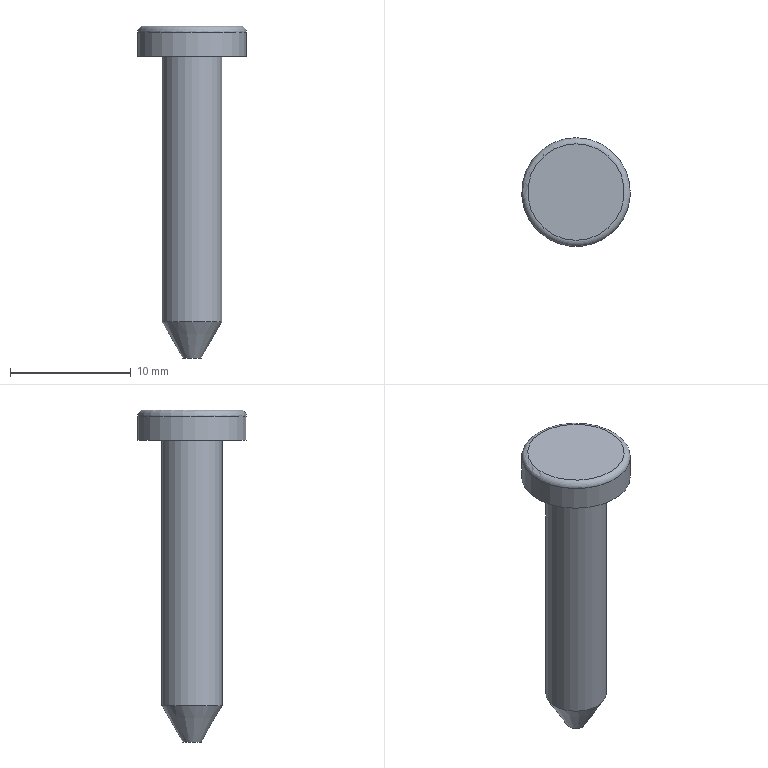Part | STEP file | 1-40.5 | 1 solid | 7 faces | box 9 x 9 x 27.5 mm | volume 617.052 mm3 | plane 3 | cylinder 2 | cone 1 | torus 1 | commonest cylinder face diameters 5 x1 9 x1
STEP:
#1=CARTESIAN_POINT('',(0.,0.,0.));
#2=DIRECTION('',(0.,0.,1.));
#3=DIRECTION('',(1.,0.,0.));
#4=AXIS2_PLACEMENT_3D('',#1,#2,#3);
#5=CARTESIAN_POINT('',(0.,4.5,0.));
#6=VERTEX_POINT('',#5);
#7=CARTESIAN_POINT('',(0.,0.,0.));
#8=DIRECTION('',(0.,0.,1.));
#9=DIRECTION('',(0.,1.,0.));
#10=AXIS2_PLACEMENT_3D('',#7,#8,#9);
#11=CIRCLE('',#10,4.5);
#12=CARTESIAN_POINT('',(0.,-1.206,0.));
#13=DIRECTION('',(0.,0.,1.));
#14=DIRECTION('',(1.,0.,0.));
#15=AXIS2_PLACEMENT_3D('',#12,#13,#14);
#16=PLANE('',#15);
#17=CARTESIAN_POINT('',(0.,1.206));
#18=DIRECTION('',(0.,1.));
#19=AXIS2_PLACEMENT_2D('',#17,#18);
#20=CIRCLE('',#19,4.5);
#21=(GEOMETRIC_REPRESENTATION_CONTEXT(2)PARAMETRIC_REPRESENTATION_CONTEXT()REPRESENTATION_CONTEXT('',''));
#22=DEFINITIONAL_REPRESENTATION('',(#20),#21);
#23=PCURVE('',#16,#22);
#24=CARTESIAN_POINT('',(0.,0.,0.));
#25=DIRECTION('',(0.,0.,1.));
#26=DIRECTION('',(0.,1.,0.));
#27=AXIS2_PLACEMENT_3D('',#24,#25,#26);
#28=CYLINDRICAL_SURFACE('',#27,4.5);
#29=CARTESIAN_POINT('',(0.,0.));
#30=DIRECTION('',(1.,0.));
#31=VECTOR('',#30,1.);
#32=LINE('',#29,#31);
#33=(GEOMETRIC_REPRESENTATION_CONTEXT(2)PARAMETRIC_REPRESENTATION_CONTEXT()REPRESENTATION_CONTEXT('',''));
#34=DEFINITIONAL_REPRESENTATION('',(#32),#33);
#35=PCURVE('',#28,#34);
#36=SURFACE_CURVE('',#11,(#23,#35),.PCURVE_S1.);
#37=EDGE_CURVE('',#6,#6,#36,.T.);
#38=ORIENTED_EDGE('',*,*,#37,.T.);
#39=EDGE_LOOP('',(#38));
#40=FACE_BOUND('',#39,.F.);
#41=CARTESIAN_POINT('',(0.,2.5,0.));
#42=VERTEX_POINT('',#41);
#43=CARTESIAN_POINT('',(0.,0.,0.));
#44=DIRECTION('',(0.,0.,1.));
#45=DIRECTION('',(0.,1.,0.));
#46=AXIS2_PLACEMENT_3D('',#43,#44,#45);
#47=CIRCLE('',#46,2.5);
#48=CARTESIAN_POINT('',(0.,1.206));
#49=DIRECTION('',(0.,1.));
#50=AXIS2_PLACEMENT_2D('',#48,#49);
#51=CIRCLE('',#50,2.5);
#52=(GEOMETRIC_REPRESENTATION_CONTEXT(2)PARAMETRIC_REPRESENTATION_CONTEXT()REPRESENTATION_CONTEXT('',''));
#53=DEFINITIONAL_REPRESENTATION('',(#51),#52);
#54=PCURVE('',#16,#53);
#55=CARTESIAN_POINT('',(0.,0.,0.));
#56=DIRECTION('',(0.,0.,-1.));
#57=DIRECTION('',(0.,1.,0.));
#58=AXIS2_PLACEMENT_3D('',#55,#56,#57);
#59=CYLINDRICAL_SURFACE('',#58,2.5);
#60=CARTESIAN_POINT('',(6.283,0.));
#61=DIRECTION('',(-1.,0.));
#62=VECTOR('',#61,1.);
#63=LINE('',#60,#62);
#64=(GEOMETRIC_REPRESENTATION_CONTEXT(2)PARAMETRIC_REPRESENTATION_CONTEXT()REPRESENTATION_CONTEXT('',''));
#65=DEFINITIONAL_REPRESENTATION('',(#63),#64);
#66=PCURVE('',#59,#65);
#67=SURFACE_CURVE('',#47,(#54,#66),.PCURVE_S1.);
#68=EDGE_CURVE('',#42,#42,#67,.T.);
#69=ORIENTED_EDGE('',*,*,#68,.F.);
#70=EDGE_LOOP('',(#69));
#71=FACE_BOUND('',#70,.F.);
#72=ADVANCED_FACE('',(#40,#71),#16,.F.);
#73=CARTESIAN_POINT('',(0.,2.5,-22.));
#74=VERTEX_POINT('',#73);
#75=CARTESIAN_POINT('',(0.,2.5,0.));
#76=DIRECTION('',(0.,0.,-1.));
#77=VECTOR('',#76,1.);
#78=LINE('',#75,#77);
#79=CARTESIAN_POINT('',(6.283,0.));
#80=DIRECTION('',(0.,1.));
#81=VECTOR('',#80,1.);
#82=LINE('',#79,#81);
#83=(GEOMETRIC_REPRESENTATION_CONTEXT(2)PARAMETRIC_REPRESENTATION_CONTEXT()REPRESENTATION_CONTEXT('',''));
#84=DEFINITIONAL_REPRESENTATION('',(#82),#83);
#85=PCURVE('',#59,#84);
#86=CARTESIAN_POINT('',(0.,0.));
#87=DIRECTION('',(0.,1.));
#88=VECTOR('',#87,1.);
#89=LINE('',#86,#88);
#90=(GEOMETRIC_REPRESENTATION_CONTEXT(2)PARAMETRIC_REPRESENTATION_CONTEXT()REPRESENTATION_CONTEXT('',''));
#91=DEFINITIONAL_REPRESENTATION('',(#89),#90);
#92=PCURVE('',#59,#91);
#93=SEAM_CURVE('',#78,(#85,#92),.PCURVE_S1.);
#94=EDGE_CURVE('',#42,#74,#93,.T.);
#95=ORIENTED_EDGE('',*,*,#94,.T.);
#96=CARTESIAN_POINT('',(0.,0.,-22.));
#97=DIRECTION('',(0.,0.,1.));
#98=DIRECTION('',(0.,1.,0.));
#99=AXIS2_PLACEMENT_3D('',#96,#97,#98);
#100=CIRCLE('',#99,2.5);
#101=CARTESIAN_POINT('',(6.283,22.));
#102=DIRECTION('',(-1.,0.));
#103=VECTOR('',#102,1.);
#104=LINE('',#101,#103);
#105=(GEOMETRIC_REPRESENTATION_CONTEXT(2)PARAMETRIC_REPRESENTATION_CONTEXT()REPRESENTATION_CONTEXT('',''));
#106=DEFINITIONAL_REPRESENTATION('',(#104),#105);
#107=PCURVE('',#59,#106);
#108=CARTESIAN_POINT('',(0.,0.,-25.));
#109=DIRECTION('',(0.,0.,1.));
#110=DIRECTION('',(0.,1.,0.));
#111=AXIS2_PLACEMENT_3D('',#108,#109,#110);
#112=CONICAL_SURFACE('',#111,0.7679,0.5236);
#113=CARTESIAN_POINT('',(0.,3.));
#114=DIRECTION('',(1.,0.));
#115=VECTOR('',#114,1.);
#116=LINE('',#113,#115);
#117=(GEOMETRIC_REPRESENTATION_CONTEXT(2)PARAMETRIC_REPRESENTATION_CONTEXT()REPRESENTATION_CONTEXT('',''));
#118=DEFINITIONAL_REPRESENTATION('',(#116),#117);
#119=PCURVE('',#112,#118);
#120=SURFACE_CURVE('',#100,(#107,#119),.PCURVE_S1.);
#121=EDGE_CURVE('',#74,#74,#120,.T.);
#122=ORIENTED_EDGE('',*,*,#121,.T.);
#123=ORIENTED_EDGE('',*,*,#94,.F.);
#124=ORIENTED_EDGE('',*,*,#68,.F.);
#125=EDGE_LOOP('',(#95,#122,#123,#124));
#126=FACE_BOUND('',#125,.T.);
#127=ADVANCED_FACE('',(#126),#59,.T.);
#128=CARTESIAN_POINT('',(0.,0.7679,-25.));
#129=VERTEX_POINT('',#128);
#130=CARTESIAN_POINT('',(0.,0.7679,-25.));
#131=DIRECTION('',(0.,0.5,0.866));
#132=VECTOR('',#131,1.);
#133=LINE('',#130,#132);
#134=CARTESIAN_POINT('',(6.283,0.));
#135=CARTESIAN_POINT('',(6.283,0.04545));
#136=CARTESIAN_POINT('',(6.283,0.1364));
#137=CARTESIAN_POINT('',(6.283,0.2727));
#138=CARTESIAN_POINT('',(6.283,0.4091));
#139=CARTESIAN_POINT('',(6.283,0.5455));
#140=CARTESIAN_POINT('',(6.283,0.6818));
#141=CARTESIAN_POINT('',(6.283,0.8182));
#142=CARTESIAN_POINT('',(6.283,0.9545));
#143=CARTESIAN_POINT('',(6.283,1.091));
#144=CARTESIAN_POINT('',(6.283,1.227));
#145=CARTESIAN_POINT('',(6.283,1.364));
#146=CARTESIAN_POINT('',(6.283,1.5));
#147=CARTESIAN_POINT('',(6.283,1.636));
#148=CARTESIAN_POINT('',(6.283,1.773));
#149=CARTESIAN_POINT('',(6.283,1.909));
#150=CARTESIAN_POINT('',(6.283,2.045));
#151=CARTESIAN_POINT('',(6.283,2.182));
#152=CARTESIAN_POINT('',(6.283,2.318));
#153=CARTESIAN_POINT('',(6.283,2.455));
#154=CARTESIAN_POINT('',(6.283,2.591));
#155=CARTESIAN_POINT('',(6.283,2.727));
#156=CARTESIAN_POINT('',(6.283,2.864));
#157=CARTESIAN_POINT('',(6.283,2.955));
#158=CARTESIAN_POINT('',(6.283,3.));
#159=B_SPLINE_CURVE_WITH_KNOTS('',3,(#134,#135,#136,#137,#138,#139,#140,#141,#142,#143,#144,#145,#146,#147,#148,#149,#150,#151,#152,#153,#154,#155,#156,#157,#158),.UNSPECIFIED.,.F.,.F.,(4,1,1,1,1,1,1,1,1,1,1,1,1,1,1,1,1,1,1,1,1,1,4),(0.,0.1575,0.3149,0.4724,0.6298,0.7873,0.9448,1.102,1.26,1.417,1.575,1.732,1.89,2.047,2.204,2.362,2.519,2.677,2.834,2.992,3.149,3.307,3.464),.QUASI_UNIFORM_KNOTS.);
#160=(GEOMETRIC_REPRESENTATION_CONTEXT(2)PARAMETRIC_REPRESENTATION_CONTEXT()REPRESENTATION_CONTEXT('',''));
#161=DEFINITIONAL_REPRESENTATION('',(#159),#160);
#162=PCURVE('',#112,#161);
#163=CARTESIAN_POINT('',(0.,0.));
#164=CARTESIAN_POINT('',(0.,0.04545));
#165=CARTESIAN_POINT('',(0.,0.1364));
#166=CARTESIAN_POINT('',(0.,0.2727));
#167=CARTESIAN_POINT('',(0.,0.4091));
#168=CARTESIAN_POINT('',(0.,0.5455));
#169=CARTESIAN_POINT('',(0.,0.6818));
#170=CARTESIAN_POINT('',(0.,0.8182));
#171=CARTESIAN_POINT('',(0.,0.9545));
#172=CARTESIAN_POINT('',(0.,1.091));
#173=CARTESIAN_POINT('',(0.,1.227));
#174=CARTESIAN_POINT('',(0.,1.364));
#175=CARTESIAN_POINT('',(0.,1.5));
#176=CARTESIAN_POINT('',(0.,1.636));
#177=CARTESIAN_POINT('',(0.,1.773));
#178=CARTESIAN_POINT('',(0.,1.909));
#179=CARTESIAN_POINT('',(0.,2.045));
#180=CARTESIAN_POINT('',(0.,2.182));
#181=CARTESIAN_POINT('',(0.,2.318));
#182=CARTESIAN_POINT('',(0.,2.455));
#183=CARTESIAN_POINT('',(0.,2.591));
#184=CARTESIAN_POINT('',(0.,2.727));
#185=CARTESIAN_POINT('',(0.,2.864));
#186=CARTESIAN_POINT('',(0.,2.955));
#187=CARTESIAN_POINT('',(0.,3.));
#188=B_SPLINE_CURVE_WITH_KNOTS('',3,(#163,#164,#165,#166,#167,#168,#169,#170,#171,#172,#173,#174,#175,#176,#177,#178,#179,#180,#181,#182,#183,#184,#185,#186,#187),.UNSPECIFIED.,.F.,.F.,(4,1,1,1,1,1,1,1,1,1,1,1,1,1,1,1,1,1,1,1,1,1,4),(0.,0.1575,0.3149,0.4724,0.6298,0.7873,0.9448,1.102,1.26,1.417,1.575,1.732,1.89,2.047,2.204,2.362,2.519,2.677,2.834,2.992,3.149,3.307,3.464),.QUASI_UNIFORM_KNOTS.);
#189=(GEOMETRIC_REPRESENTATION_CONTEXT(2)PARAMETRIC_REPRESENTATION_CONTEXT()REPRESENTATION_CONTEXT('',''));
#190=DEFINITIONAL_REPRESENTATION('',(#188),#189);
#191=PCURVE('',#112,#190);
#192=SEAM_CURVE('',#133,(#162,#191),.PCURVE_S1.);
#193=EDGE_CURVE('',#129,#74,#192,.T.);
#194=ORIENTED_EDGE('',*,*,#193,.T.);
#195=ORIENTED_EDGE('',*,*,#121,.F.);
#196=ORIENTED_EDGE('',*,*,#193,.F.);
#197=CARTESIAN_POINT('',(0.,0.,-25.));
#198=DIRECTION('',(0.,0.,-1.));
#199=DIRECTION('',(0.,1.,0.));
#200=AXIS2_PLACEMENT_3D('',#197,#198,#199);
#201=CIRCLE('',#200,0.7679);
#202=CARTESIAN_POINT('',(6.283,0.));
#203=DIRECTION('',(-1.,0.));
#204=VECTOR('',#203,1.);
#205=LINE('',#202,#204);
#206=(GEOMETRIC_REPRESENTATION_CONTEXT(2)PARAMETRIC_REPRESENTATION_CONTEXT()REPRESENTATION_CONTEXT('',''));
#207=DEFINITIONAL_REPRESENTATION('',(#205),#206);
#208=PCURVE('',#112,#207);
#209=CARTESIAN_POINT('',(0.,0.,-25.));
#210=DIRECTION('',(0.,0.,-1.));
#211=DIRECTION('',(0.,1.,0.));
#212=AXIS2_PLACEMENT_3D('',#209,#210,#211);
#213=PLANE('',#212);
#214=CARTESIAN_POINT('',(0.,0.));
#215=DIRECTION('',(1.,0.));
#216=AXIS2_PLACEMENT_2D('',#214,#215);
#217=CIRCLE('',#216,0.7679);
#218=(GEOMETRIC_REPRESENTATION_CONTEXT(2)PARAMETRIC_REPRESENTATION_CONTEXT()REPRESENTATION_CONTEXT('',''));
#219=DEFINITIONAL_REPRESENTATION('',(#217),#218);
#220=PCURVE('',#213,#219);
#221=SURFACE_CURVE('',#201,(#208,#220),.PCURVE_S1.);
#222=EDGE_CURVE('',#129,#129,#221,.T.);
#223=ORIENTED_EDGE('',*,*,#222,.F.);
#224=EDGE_LOOP('',(#194,#195,#196,#223));
#225=FACE_BOUND('',#224,.T.);
#226=ADVANCED_FACE('',(#225),#112,.T.);
#227=ORIENTED_EDGE('',*,*,#222,.T.);
#228=EDGE_LOOP('',(#227));
#229=FACE_BOUND('',#228,.T.);
#230=ADVANCED_FACE('',(#229),#213,.T.);
#231=CARTESIAN_POINT('',(0.,4.,2.5));
#232=VERTEX_POINT('',#231);
#233=CARTESIAN_POINT('',(0.,0.,2.5));
#234=DIRECTION('',(0.,0.,-1.));
#235=DIRECTION('',(0.,1.,0.));
#236=AXIS2_PLACEMENT_3D('',#233,#234,#235);
#237=CIRCLE('',#236,4.);
#238=CARTESIAN_POINT('',(0.,-1.206,2.5));
#239=DIRECTION('',(0.,0.,1.));
#240=DIRECTION('',(1.,0.,0.));
#241=AXIS2_PLACEMENT_3D('',#238,#239,#240);
#242=PLANE('',#241);
#243=CARTESIAN_POINT('',(0.,5.206));
#244=CARTESIAN_POINT('',(6.928,5.206));
#245=CARTESIAN_POINT('',(3.464,-0.7942));
#246=CARTESIAN_POINT('',(0.,-6.794));
#247=CARTESIAN_POINT('',(-3.464,-0.7942));
#248=CARTESIAN_POINT('',(-6.928,5.206));
#249=CARTESIAN_POINT('',(0.,5.206));
#250=(BOUNDED_CURVE()B_SPLINE_CURVE(2,(#243,#244,#245,#246,#247,#248,#249),.UNSPECIFIED.,.T.,.F.)B_SPLINE_CURVE_WITH_KNOTS((1,2,2,2,2,1),(-2.094,0.,2.094,4.189,6.283,8.378),.UNSPECIFIED.)CURVE()GEOMETRIC_REPRESENTATION_ITEM()RATIONAL_B_SPLINE_CURVE((1.,0.5,1.,0.5,1.,0.5,1.))REPRESENTATION_ITEM(''));
#251=(GEOMETRIC_REPRESENTATION_CONTEXT(2)PARAMETRIC_REPRESENTATION_CONTEXT()REPRESENTATION_CONTEXT('',''));
#252=DEFINITIONAL_REPRESENTATION('',(#250),#251);
#253=PCURVE('',#242,#252);
#254=CARTESIAN_POINT('',(0.,0.,2.));
#255=DIRECTION('',(0.,0.,1.));
#256=DIRECTION('',(0.,1.,0.));
#257=AXIS2_PLACEMENT_3D('',#254,#255,#256);
#258=TOROIDAL_SURFACE('',#257,4.,0.5);
#259=CARTESIAN_POINT('',(6.283,1.571));
#260=DIRECTION('',(-1.,0.));
#261=VECTOR('',#260,1.);
#262=LINE('',#259,#261);
#263=(GEOMETRIC_REPRESENTATION_CONTEXT(2)PARAMETRIC_REPRESENTATION_CONTEXT()REPRESENTATION_CONTEXT('',''));
#264=DEFINITIONAL_REPRESENTATION('',(#262),#263);
#265=PCURVE('',#258,#264);
#266=SURFACE_CURVE('',#237,(#253,#265),.PCURVE_S1.);
#267=EDGE_CURVE('',#232,#232,#266,.T.);
#268=ORIENTED_EDGE('',*,*,#267,.F.);
#269=EDGE_LOOP('',(#268));
#270=FACE_BOUND('',#269,.T.);
#271=ADVANCED_FACE('',(#270),#242,.T.);
#272=ORIENTED_EDGE('',*,*,#37,.T.);
#273=CARTESIAN_POINT('',(0.,4.5,2.));
#274=VERTEX_POINT('',#273);
#275=CARTESIAN_POINT('',(0.,4.5,0.));
#276=DIRECTION('',(0.,0.,1.));
#277=VECTOR('',#276,1.);
#278=LINE('',#275,#277);
#279=CARTESIAN_POINT('',(6.283,0.));
#280=DIRECTION('',(0.,1.));
#281=VECTOR('',#280,1.);
#282=LINE('',#279,#281);
#283=(GEOMETRIC_REPRESENTATION_CONTEXT(2)PARAMETRIC_REPRESENTATION_CONTEXT()REPRESENTATION_CONTEXT('',''));
#284=DEFINITIONAL_REPRESENTATION('',(#282),#283);
#285=PCURVE('',#28,#284);
#286=CARTESIAN_POINT('',(0.,0.));
#287=DIRECTION('',(0.,1.));
#288=VECTOR('',#287,1.);
#289=LINE('',#286,#288);
#290=(GEOMETRIC_REPRESENTATION_CONTEXT(2)PARAMETRIC_REPRESENTATION_CONTEXT()REPRESENTATION_CONTEXT('',''));
#291=DEFINITIONAL_REPRESENTATION('',(#289),#290);
#292=PCURVE('',#28,#291);
#293=SEAM_CURVE('',#278,(#285,#292),.PCURVE_S1.);
#294=EDGE_CURVE('',#6,#274,#293,.T.);
#295=ORIENTED_EDGE('',*,*,#294,.T.);
#296=CARTESIAN_POINT('',(0.,0.,2.));
#297=DIRECTION('',(0.,0.,-1.));
#298=DIRECTION('',(0.,1.,0.));
#299=AXIS2_PLACEMENT_3D('',#296,#297,#298);
#300=CIRCLE('',#299,4.5);
#301=CARTESIAN_POINT('',(6.283,2.));
#302=DIRECTION('',(-1.,0.));
#303=VECTOR('',#302,1.);
#304=LINE('',#301,#303);
#305=(GEOMETRIC_REPRESENTATION_CONTEXT(2)PARAMETRIC_REPRESENTATION_CONTEXT()REPRESENTATION_CONTEXT('',''));
#306=DEFINITIONAL_REPRESENTATION('',(#304),#305);
#307=PCURVE('',#28,#306);
#308=CARTESIAN_POINT('',(6.283,0.));
#309=DIRECTION('',(-1.,0.));
#310=VECTOR('',#309,1.);
#311=LINE('',#308,#310);
#312=(GEOMETRIC_REPRESENTATION_CONTEXT(2)PARAMETRIC_REPRESENTATION_CONTEXT()REPRESENTATION_CONTEXT('',''));
#313=DEFINITIONAL_REPRESENTATION('',(#311),#312);
#314=PCURVE('',#258,#313);
#315=SURFACE_CURVE('',#300,(#307,#314),.PCURVE_S1.);
#316=EDGE_CURVE('',#274,#274,#315,.T.);
#317=ORIENTED_EDGE('',*,*,#316,.T.);
#318=ORIENTED_EDGE('',*,*,#294,.F.);
#319=EDGE_LOOP('',(#272,#295,#317,#318));
#320=FACE_BOUND('',#319,.T.);
#321=ADVANCED_FACE('',(#320),#28,.T.);
#322=CARTESIAN_POINT('',(0.,4.,2.));
#323=DIRECTION('',(-1.,0.,0.));
#324=DIRECTION('',(0.,0.,1.));
#325=AXIS2_PLACEMENT_3D('',#322,#323,#324);
#326=CIRCLE('',#325,0.5);
#327=CARTESIAN_POINT('',(0.,1.571));
#328=CARTESIAN_POINT('',(0.,1.547));
#329=CARTESIAN_POINT('',(0.,1.499));
#330=CARTESIAN_POINT('',(0.,1.428));
#331=CARTESIAN_POINT('',(0.,1.357));
#332=CARTESIAN_POINT('',(0.,1.285));
#333=CARTESIAN_POINT('',(0.,1.214));
#334=CARTESIAN_POINT('',(0.,1.142));
#335=CARTESIAN_POINT('',(0.,1.071));
#336=CARTESIAN_POINT('',(0.,0.9996));
#337=CARTESIAN_POINT('',(0.,0.9282));
#338=CARTESIAN_POINT('',(0.,0.8568));
#339=CARTESIAN_POINT('',(0.,0.7854));
#340=CARTESIAN_POINT('',(0.,0.714));
#341=CARTESIAN_POINT('',(0.,0.6426));
#342=CARTESIAN_POINT('',(0.,0.5712));
#343=CARTESIAN_POINT('',(0.,0.4998));
#344=CARTESIAN_POINT('',(0.,0.4284));
#345=CARTESIAN_POINT('',(0.,0.357));
#346=CARTESIAN_POINT('',(0.,0.2856));
#347=CARTESIAN_POINT('',(0.,0.2142));
#348=CARTESIAN_POINT('',(0.,0.1428));
#349=CARTESIAN_POINT('',(0.,0.0714));
#350=CARTESIAN_POINT('',(0.,0.0238));
#351=CARTESIAN_POINT('',(0.,0.));
#352=B_SPLINE_CURVE_WITH_KNOTS('',3,(#327,#328,#329,#330,#331,#332,#333,#334,#335,#336,#337,#338,#339,#340,#341,#342,#343,#344,#345,#346,#347,#348,#349,#350,#351),.UNSPECIFIED.,.F.,.F.,(4,1,1,1,1,1,1,1,1,1,1,1,1,1,1,1,1,1,1,1,1,1,4),(0.,0.0714,0.1428,0.2142,0.2856,0.357,0.4284,0.4998,0.5712,0.6426,0.714,0.7854,0.8568,0.9282,0.9996,1.071,1.142,1.214,1.285,1.357,1.428,1.499,1.571),.QUASI_UNIFORM_KNOTS.);
#353=(GEOMETRIC_REPRESENTATION_CONTEXT(2)PARAMETRIC_REPRESENTATION_CONTEXT()REPRESENTATION_CONTEXT('',''));
#354=DEFINITIONAL_REPRESENTATION('',(#352),#353);
#355=PCURVE('',#258,#354);
#356=CARTESIAN_POINT('',(6.283,1.571));
#357=CARTESIAN_POINT('',(6.283,1.547));
#358=CARTESIAN_POINT('',(6.283,1.499));
#359=CARTESIAN_POINT('',(6.283,1.428));
#360=CARTESIAN_POINT('',(6.283,1.357));
#361=CARTESIAN_POINT('',(6.283,1.285));
#362=CARTESIAN_POINT('',(6.283,1.214));
#363=CARTESIAN_POINT('',(6.283,1.142));
#364=CARTESIAN_POINT('',(6.283,1.071));
#365=CARTESIAN_POINT('',(6.283,0.9996));
#366=CARTESIAN_POINT('',(6.283,0.9282));
#367=CARTESIAN_POINT('',(6.283,0.8568));
#368=CARTESIAN_POINT('',(6.283,0.7854));
#369=CARTESIAN_POINT('',(6.283,0.714));
#370=CARTESIAN_POINT('',(6.283,0.6426));
#371=CARTESIAN_POINT('',(6.283,0.5712));
#372=CARTESIAN_POINT('',(6.283,0.4998));
#373=CARTESIAN_POINT('',(6.283,0.4284));
#374=CARTESIAN_POINT('',(6.283,0.357));
#375=CARTESIAN_POINT('',(6.283,0.2856));
#376=CARTESIAN_POINT('',(6.283,0.2142));
#377=CARTESIAN_POINT('',(6.283,0.1428));
#378=CARTESIAN_POINT('',(6.283,0.0714));
#379=CARTESIAN_POINT('',(6.283,0.0238));
#380=CARTESIAN_POINT('',(6.283,0.));
#381=B_SPLINE_CURVE_WITH_KNOTS('',3,(#356,#357,#358,#359,#360,#361,#362,#363,#364,#365,#366,#367,#368,#369,#370,#371,#372,#373,#374,#375,#376,#377,#378,#379,#380),.UNSPECIFIED.,.F.,.F.,(4,1,1,1,1,1,1,1,1,1,1,1,1,1,1,1,1,1,1,1,1,1,4),(0.,0.0714,0.1428,0.2142,0.2856,0.357,0.4284,0.4998,0.5712,0.6426,0.714,0.7854,0.8568,0.9282,0.9996,1.071,1.142,1.214,1.285,1.357,1.428,1.499,1.571),.QUASI_UNIFORM_KNOTS.);
#382=(GEOMETRIC_REPRESENTATION_CONTEXT(2)PARAMETRIC_REPRESENTATION_CONTEXT()REPRESENTATION_CONTEXT('',''));
#383=DEFINITIONAL_REPRESENTATION('',(#381),#382);
#384=PCURVE('',#258,#383);
#385=SEAM_CURVE('',#326,(#355,#384),.PCURVE_S1.);
#386=EDGE_CURVE('',#232,#274,#385,.T.);
#387=ORIENTED_EDGE('',*,*,#386,.T.);
#388=ORIENTED_EDGE('',*,*,#316,.F.);
#389=ORIENTED_EDGE('',*,*,#386,.F.);
#390=ORIENTED_EDGE('',*,*,#267,.T.);
#391=EDGE_LOOP('',(#387,#388,#389,#390));
#392=FACE_BOUND('',#391,.T.);
#393=ADVANCED_FACE('',(#392),#258,.T.);
#394=CLOSED_SHELL('',(#72,#127,#226,#230,#271,#321,#393));
#395=MANIFOLD_SOLID_BREP('',#394);
#396=(LENGTH_UNIT()NAMED_UNIT(*)SI_UNIT(.MILLI.,.METRE.));
#397=UNCERTAINTY_MEASURE_WITH_UNIT(LENGTH_MEASURE(0.0000001),#396,'','');
#398=(NAMED_UNIT(*)PLANE_ANGLE_UNIT()SI_UNIT($,.RADIAN.));
#399=(NAMED_UNIT(*)SI_UNIT($,.STERADIAN.)SOLID_ANGLE_UNIT());
#400=(GEOMETRIC_REPRESENTATION_CONTEXT(3)GLOBAL_UNCERTAINTY_ASSIGNED_CONTEXT((#397))GLOBAL_UNIT_ASSIGNED_CONTEXT((#396,#398,#399))REPRESENTATION_CONTEXT('',''));
#401=ADVANCED_BREP_SHAPE_REPRESENTATION('',(#4,#395),#400);